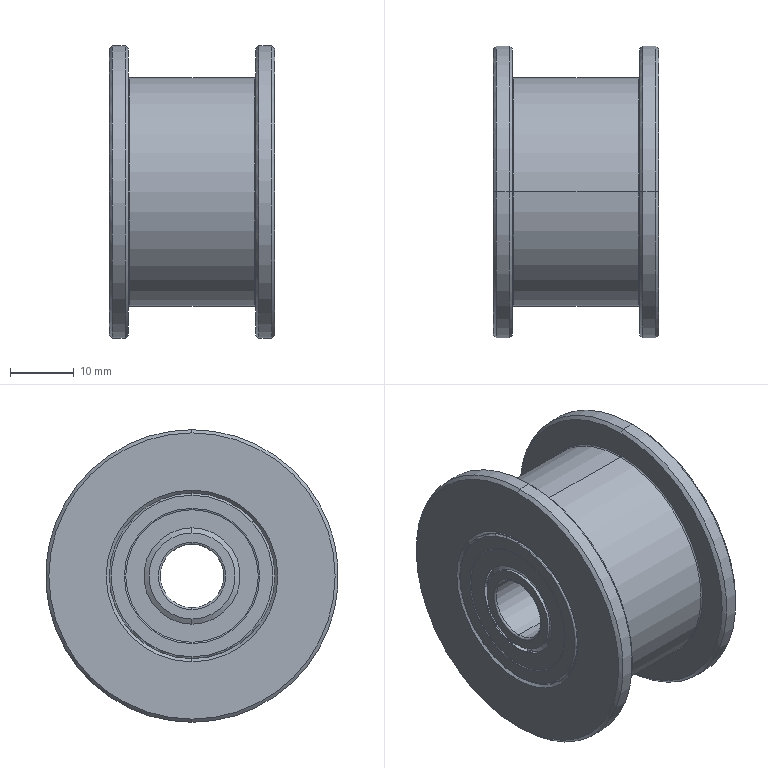Part | SolidWorks | 27 solids | 366 faces | box 26 x 46 x 46 mm | volume 23618 mm3 | cylinder 128 | sphere 96 | plane 66 | torus 52 | cone 24 | commonest cylinder face diameters 17.2 x42 18.8 x42 13.556 x8 15.333 x8 20.667 x8 26 x8